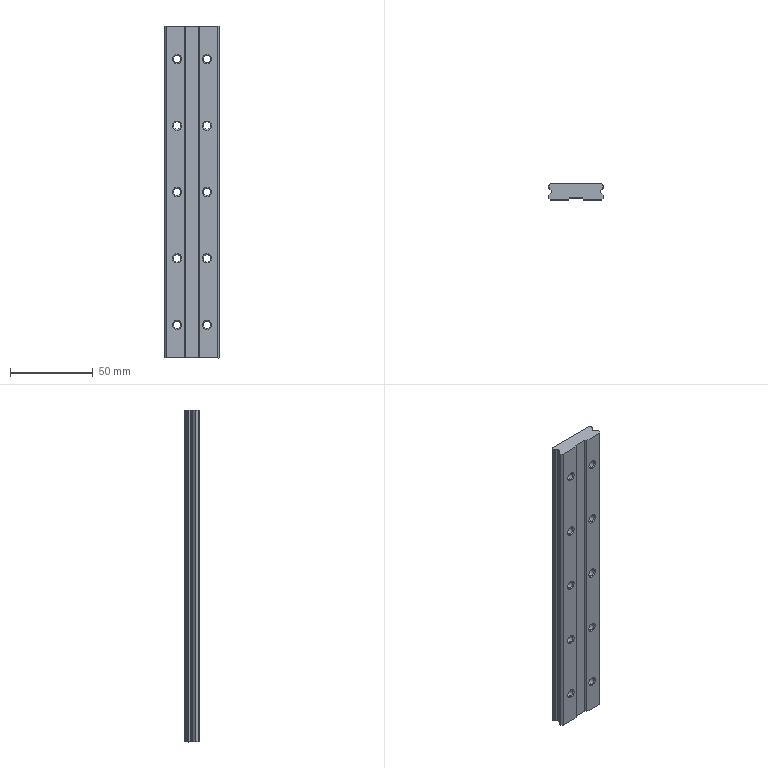Part | SolidWorks | features BaseBody 1 | 1 solid | 132 faces | box 33 x 9.3 x 200 mm | volume 53846 mm3 | cylinder 56 | cone 40 | plane 36 | commonest cylinder face diameters 4.5 x20 8 x20 1 x10 0.77 x6